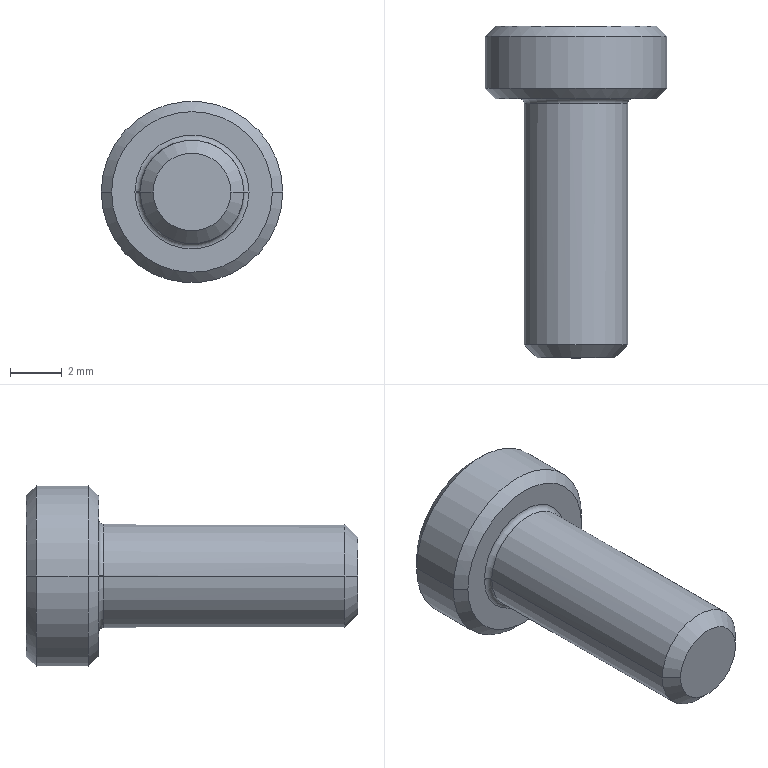Part | SolidWorks | features BaseBody 1 | 1 solid | 32 faces | box 7 x 12.8 x 7 mm | volume 210.469 mm3 | cylinder 18 | cone 6 | plane 4 | torus 4 | commonest cylinder face diameters 1 x8 3.286 x6 4 x2 7 x2
STEP:
#1=CARTESIAN_POINT('',(1970.222,195.3,831.468));
#2=VERTEX_POINT('',#1);
#3=CARTESIAN_POINT('',(1964.022,195.3,831.468));
#4=VERTEX_POINT('',#3);
#5=CARTESIAN_POINT('',(1970.222,195.3,831.468));
#6=CARTESIAN_POINT('',(1970.222,195.3,831.123));
#7=CARTESIAN_POINT('',(1970.174,195.3,830.778));
#8=CARTESIAN_POINT('',(1970.078,195.3,830.441));
#9=CARTESIAN_POINT('',(1969.795,195.3,829.805));
#10=CARTESIAN_POINT('',(1969.349,195.3,829.27));
#11=CARTESIAN_POINT('',(1969.09,195.3,829.035));
#12=CARTESIAN_POINT('',(1968.513,195.3,828.644));
#13=CARTESIAN_POINT('',(1967.852,195.3,828.425));
#14=CARTESIAN_POINT('',(1967.508,195.3,828.362));
#15=CARTESIAN_POINT('',(1966.811,195.3,828.335));
#16=CARTESIAN_POINT('',(1966.134,195.3,828.498));
#17=CARTESIAN_POINT('',(1965.809,195.3,828.627));
#18=CARTESIAN_POINT('',(1965.204,195.3,828.971));
#19=CARTESIAN_POINT('',(1964.715,195.3,829.468));
#20=CARTESIAN_POINT('',(1964.507,195.3,829.749));
#21=CARTESIAN_POINT('',(1964.233,195.3,830.253));
#22=CARTESIAN_POINT('',(1964.082,195.3,830.802));
#23=CARTESIAN_POINT('',(1964.042,195.3,831.022));
#24=CARTESIAN_POINT('',(1964.022,195.3,831.245));
#25=CARTESIAN_POINT('',(1964.022,195.3,831.468));
#26=B_SPLINE_CURVE_WITH_KNOTS('',5,(#5,#6,#7,#8,#9,#10,#11,#12,#13,#14,#15,#16,#17,#18,#19,#20,#21,#22,#23,#24,#25),.UNSPECIFIED.,.F.,.F.,(6,3,3,3,3,3,6),(0.,0.1771,0.3543,0.5314,0.7085,0.8857,1.),.UNSPECIFIED.);
#27=EDGE_CURVE('',#2,#4,#26,.T.);
#28=ORIENTED_EDGE('',*,*,#27,.F.);
#29=CARTESIAN_POINT('',(1967.122,195.3,831.468));
#30=DIRECTION('',(0.,-1.,0.));
#31=DIRECTION('',(0.,0.,-1.));
#32=AXIS2_PLACEMENT_3D('',#29,#30,#31);
#33=CIRCLE('',#32,3.1);
#34=EDGE_CURVE('',#2,#4,#33,.T.);
#35=ORIENTED_EDGE('',*,*,#34,.T.);
#36=EDGE_LOOP('',(#28,#35));
#37=FACE_OUTER_BOUND('',#36,.T.);
#38=CARTESIAN_POINT('',(1964.922,195.3,831.495));
#39=VERTEX_POINT('',#38);
#40=CARTESIAN_POINT('',(1964.922,195.3,831.468));
#41=VERTEX_POINT('',#40);
#42=CARTESIAN_POINT('',(1967.122,195.3,831.468));
#43=DIRECTION('',(0.,-1.,0.));
#44=DIRECTION('',(0.,0.,-1.));
#45=AXIS2_PLACEMENT_3D('',#42,#43,#44);
#46=CIRCLE('',#45,2.2);
#47=EDGE_CURVE('',#39,#41,#46,.T.);
#48=ORIENTED_EDGE('',*,*,#47,.F.);
#49=CARTESIAN_POINT('',(1969.322,195.3,831.468));
#50=VERTEX_POINT('',#49);
#51=CARTESIAN_POINT('',(1967.122,195.3,831.468));
#52=DIRECTION('',(0.,-1.,0.));
#53=DIRECTION('',(0.,0.,-1.));
#54=AXIS2_PLACEMENT_3D('',#51,#52,#53);
#55=CIRCLE('',#54,2.2);
#56=EDGE_CURVE('',#50,#39,#55,.T.);
#57=ORIENTED_EDGE('',*,*,#56,.F.);
#58=CARTESIAN_POINT('',(1969.321,195.3,831.44));
#59=VERTEX_POINT('',#58);
#60=CARTESIAN_POINT('',(1967.122,195.3,831.468));
#61=DIRECTION('',(0.,-1.,0.));
#62=DIRECTION('',(0.,0.,-1.));
#63=AXIS2_PLACEMENT_3D('',#60,#61,#62);
#64=CIRCLE('',#63,2.2);
#65=EDGE_CURVE('',#59,#50,#64,.T.);
#66=ORIENTED_EDGE('',*,*,#65,.F.);
#67=CARTESIAN_POINT('',(1967.122,195.3,831.468));
#68=DIRECTION('',(0.,-1.,0.));
#69=DIRECTION('',(0.,0.,-1.));
#70=AXIS2_PLACEMENT_3D('',#67,#68,#69);
#71=CIRCLE('',#70,2.2);
#72=EDGE_CURVE('',#41,#59,#71,.T.);
#73=ORIENTED_EDGE('',*,*,#72,.F.);
#74=EDGE_LOOP('',(#48,#57,#66,#73));
#75=FACE_BOUND('',#74,.T.);
#76=CARTESIAN_POINT('',(1967.122,195.3,831.468));
#77=DIRECTION('',(0.,-1.,0.));
#78=DIRECTION('',(1.,0.,0.));
#79=AXIS2_PLACEMENT_3D('',#76,#77,#78);
#80=PLANE('',#79);
#81=ADVANCED_FACE('',(#37,#75),#80,.T.);
#82=CARTESIAN_POINT('',(1970.622,195.7,831.468));
#83=VERTEX_POINT('',#82);
#84=CARTESIAN_POINT('',(355522.162,353747.241,831.468));
#85=DIRECTION('',(0.7071,0.7071,0.));
#86=VECTOR('',#85,1000.);
#87=LINE('',#84,#86);
#88=EDGE_CURVE('',#2,#83,#87,.T.);
#89=ORIENTED_EDGE('',*,*,#88,.F.);
#90=ORIENTED_EDGE('',*,*,#27,.T.);
#91=CARTESIAN_POINT('',(1963.622,195.7,831.468));
#92=VERTEX_POINT('',#91);
#93=CARTESIAN_POINT('',(-351587.919,353747.241,831.468));
#94=DIRECTION('',(0.7071,-0.7071,0.));
#95=VECTOR('',#94,1000.);
#96=LINE('',#93,#95);
#97=EDGE_CURVE('',#92,#4,#96,.T.);
#98=ORIENTED_EDGE('',*,*,#97,.F.);
#99=CARTESIAN_POINT('',(1967.122,195.7,831.468));
#100=DIRECTION('',(0.,1.,0.));
#101=DIRECTION('',(0.,0.,1.));
#102=AXIS2_PLACEMENT_3D('',#99,#100,#101);
#103=CIRCLE('',#102,3.5);
#104=EDGE_CURVE('',#83,#92,#103,.T.);
#105=ORIENTED_EDGE('',*,*,#104,.F.);
#106=EDGE_LOOP('',(#89,#90,#98,#105));
#107=FACE_OUTER_BOUND('',#106,.T.);
#108=CARTESIAN_POINT('',(1967.122,195.5,831.468));
#109=DIRECTION('',(0.,1.,0.));
#110=DIRECTION('',(-1.,0.,0.));
#111=AXIS2_PLACEMENT_3D('',#108,#109,#110);
#112=CONICAL_SURFACE('',#111,3.3,0.7854);
#113=ADVANCED_FACE('',(#107),#112,.T.);
#114=ORIENTED_EDGE('',*,*,#97,.T.);
#115=ORIENTED_EDGE('',*,*,#34,.F.);
#116=ORIENTED_EDGE('',*,*,#88,.T.);
#117=CARTESIAN_POINT('',(1967.122,195.7,831.468));
#118=DIRECTION('',(0.,-1.,0.));
#119=DIRECTION('',(0.,0.,1.));
#120=AXIS2_PLACEMENT_3D('',#117,#118,#119);
#121=CIRCLE('',#120,3.5);
#122=EDGE_CURVE('',#83,#92,#121,.T.);
#123=ORIENTED_EDGE('',*,*,#122,.T.);
#124=EDGE_LOOP('',(#114,#115,#116,#123));
#125=FACE_OUTER_BOUND('',#124,.T.);
#126=CARTESIAN_POINT('',(1967.122,195.5,831.468));
#127=DIRECTION('',(0.,1.,0.));
#128=DIRECTION('',(1.,0.,0.));
#129=AXIS2_PLACEMENT_3D('',#126,#127,#128);
#130=CONICAL_SURFACE('',#129,3.3,0.7854);
#131=ADVANCED_FACE('',(#125),#130,.T.);
#132=ORIENTED_EDGE('',*,*,#47,.T.);
#133=CARTESIAN_POINT('',(1965.122,195.1,831.468));
#134=VERTEX_POINT('',#133);
#135=CARTESIAN_POINT('',(1964.922,195.1,831.468));
#136=DIRECTION('',(0.,0.,-1.));
#137=DIRECTION('',(0.,-1.,0.));
#138=AXIS2_PLACEMENT_3D('',#135,#136,#137);
#139=CIRCLE('',#138,0.2);
#140=EDGE_CURVE('',#41,#134,#139,.T.);
#141=ORIENTED_EDGE('',*,*,#140,.T.);
#142=CARTESIAN_POINT('',(1965.122,195.1,831.492));
#143=VERTEX_POINT('',#142);
#144=CARTESIAN_POINT('',(1967.122,195.1,831.468));
#145=DIRECTION('',(0.,-1.,0.));
#146=DIRECTION('',(0.,0.,-1.));
#147=AXIS2_PLACEMENT_3D('',#144,#145,#146);
#148=CIRCLE('',#147,2.);
#149=EDGE_CURVE('',#143,#134,#148,.T.);
#150=ORIENTED_EDGE('',*,*,#149,.F.);
#151=CARTESIAN_POINT('',(1964.922,195.1,831.495));
#152=DIRECTION('',(0.01244,0.,0.9999));
#153=DIRECTION('',(0.,-1.,0.));
#154=AXIS2_PLACEMENT_3D('',#151,#152,#153);
#155=CIRCLE('',#154,0.2);
#156=EDGE_CURVE('',#143,#39,#155,.T.);
#157=ORIENTED_EDGE('',*,*,#156,.T.);
#158=EDGE_LOOP('',(#132,#141,#150,#157));
#159=FACE_OUTER_BOUND('',#158,.T.);
#160=CARTESIAN_POINT('',(1967.122,195.1,831.468));
#161=DIRECTION('',(0.,-1.,0.));
#162=DIRECTION('',(0.9999,0.,-0.01244));
#163=AXIS2_PLACEMENT_3D('',#160,#161,#162);
#164=TOROIDAL_SURFACE('',#163,2.2,0.2);
#165=ADVANCED_FACE('',(#159),#164,.F.);
#166=CARTESIAN_POINT('',(1969.122,195.1,831.468));
#167=VERTEX_POINT('',#166);
#168=CARTESIAN_POINT('',(1967.122,195.1,831.468));
#169=DIRECTION('',(0.,-1.,0.));
#170=DIRECTION('',(0.,0.,-1.));
#171=AXIS2_PLACEMENT_3D('',#168,#169,#170);
#172=CIRCLE('',#171,2.);
#173=EDGE_CURVE('',#167,#143,#172,.T.);
#174=ORIENTED_EDGE('',*,*,#173,.F.);
#175=CARTESIAN_POINT('',(1969.322,195.1,831.468));
#176=DIRECTION('',(0.,0.,1.));
#177=DIRECTION('',(0.,-1.,0.));
#178=AXIS2_PLACEMENT_3D('',#175,#176,#177);
#179=CIRCLE('',#178,0.2);
#180=EDGE_CURVE('',#50,#167,#179,.T.);
#181=ORIENTED_EDGE('',*,*,#180,.F.);
#182=ORIENTED_EDGE('',*,*,#56,.T.);
#183=ORIENTED_EDGE('',*,*,#156,.F.);
#184=EDGE_LOOP('',(#174,#181,#182,#183));
#185=FACE_OUTER_BOUND('',#184,.T.);
#186=CARTESIAN_POINT('',(1967.122,195.1,831.468));
#187=DIRECTION('',(0.,-1.,0.));
#188=DIRECTION('',(-0.9999,0.,0.01244));
#189=AXIS2_PLACEMENT_3D('',#186,#187,#188);
#190=TOROIDAL_SURFACE('',#189,2.2,0.2);
#191=ADVANCED_FACE('',(#185),#190,.F.);
#192=ORIENTED_EDGE('',*,*,#65,.T.);
#193=ORIENTED_EDGE('',*,*,#180,.T.);
#194=CARTESIAN_POINT('',(1969.121,195.1,831.443));
#195=VERTEX_POINT('',#194);
#196=CARTESIAN_POINT('',(1967.122,195.1,831.468));
#197=DIRECTION('',(0.,-1.,0.));
#198=DIRECTION('',(0.,0.,-1.));
#199=AXIS2_PLACEMENT_3D('',#196,#197,#198);
#200=CIRCLE('',#199,2.);
#201=EDGE_CURVE('',#195,#167,#200,.T.);
#202=ORIENTED_EDGE('',*,*,#201,.F.);
#203=CARTESIAN_POINT('',(1969.321,195.1,831.44));
#204=DIRECTION('',(-0.01244,0.,-0.9999));
#205=DIRECTION('',(0.,-1.,0.));
#206=AXIS2_PLACEMENT_3D('',#203,#204,#205);
#207=CIRCLE('',#206,0.2);
#208=EDGE_CURVE('',#195,#59,#207,.T.);
#209=ORIENTED_EDGE('',*,*,#208,.T.);
#210=EDGE_LOOP('',(#192,#193,#202,#209));
#211=FACE_OUTER_BOUND('',#210,.T.);
#212=CARTESIAN_POINT('',(1967.122,195.1,831.468));
#213=DIRECTION('',(0.,-1.,0.));
#214=DIRECTION('',(-0.9999,0.,0.01244));
#215=AXIS2_PLACEMENT_3D('',#212,#213,#214);
#216=TOROIDAL_SURFACE('',#215,2.2,0.2);
#217=ADVANCED_FACE('',(#211),#216,.F.);
#218=CARTESIAN_POINT('',(1967.122,195.1,831.468));
#219=DIRECTION('',(0.,-1.,0.));
#220=DIRECTION('',(0.,0.,-1.));
#221=AXIS2_PLACEMENT_3D('',#218,#219,#220);
#222=CIRCLE('',#221,2.);
#223=EDGE_CURVE('',#134,#195,#222,.T.);
#224=ORIENTED_EDGE('',*,*,#223,.F.);
#225=ORIENTED_EDGE('',*,*,#140,.F.);
#226=ORIENTED_EDGE('',*,*,#72,.T.);
#227=ORIENTED_EDGE('',*,*,#208,.F.);
#228=EDGE_LOOP('',(#224,#225,#226,#227));
#229=FACE_OUTER_BOUND('',#228,.T.);
#230=CARTESIAN_POINT('',(1967.122,195.1,831.468));
#231=DIRECTION('',(0.,-1.,0.));
#232=DIRECTION('',(0.9999,0.,-0.01244));
#233=AXIS2_PLACEMENT_3D('',#230,#231,#232);
#234=TOROIDAL_SURFACE('',#233,2.2,0.2);
#235=ADVANCED_FACE('',(#229),#234,.F.);
#236=ORIENTED_EDGE('',*,*,#104,.T.);
#237=CARTESIAN_POINT('',(1963.622,197.7,831.468));
#238=VERTEX_POINT('',#237);
#239=CARTESIAN_POINT('',(1963.622,198.74,831.468));
#240=DIRECTION('',(0.,-1.,0.));
#241=VECTOR('',#240,1000.);
#242=LINE('',#239,#241);
#243=EDGE_CURVE('',#238,#92,#242,.T.);
#244=ORIENTED_EDGE('',*,*,#243,.F.);
#245=CARTESIAN_POINT('',(1970.622,197.7,831.468));
#246=VERTEX_POINT('',#245);
#247=CARTESIAN_POINT('',(1967.122,197.7,831.468));
#248=DIRECTION('',(0.,1.,0.));
#249=DIRECTION('',(0.,0.,-1.));
#250=AXIS2_PLACEMENT_3D('',#247,#248,#249);
#251=CIRCLE('',#250,3.5);
#252=EDGE_CURVE('',#246,#238,#251,.T.);
#253=ORIENTED_EDGE('',*,*,#252,.F.);
#254=CARTESIAN_POINT('',(1970.622,198.74,831.468));
#255=DIRECTION('',(0.,1.,0.));
#256=VECTOR('',#255,1000.);
#257=LINE('',#254,#256);
#258=EDGE_CURVE('',#83,#246,#257,.T.);
#259=ORIENTED_EDGE('',*,*,#258,.F.);
#260=EDGE_LOOP('',(#236,#244,#253,#259));
#261=FACE_OUTER_BOUND('',#260,.T.);
#262=CARTESIAN_POINT('',(1967.122,198.74,831.468));
#263=DIRECTION('',(0.,-1.,0.));
#264=DIRECTION('',(1.,0.,0.));
#265=AXIS2_PLACEMENT_3D('',#262,#263,#264);
#266=CYLINDRICAL_SURFACE('',#265,3.5);
#267=ADVANCED_FACE('',(#261),#266,.T.);
#268=CARTESIAN_POINT('',(1967.122,197.7,831.468));
#269=DIRECTION('',(0.,-1.,0.));
#270=DIRECTION('',(0.,0.,-1.));
#271=AXIS2_PLACEMENT_3D('',#268,#269,#270);
#272=CIRCLE('',#271,3.5);
#273=EDGE_CURVE('',#246,#238,#272,.T.);
#274=ORIENTED_EDGE('',*,*,#273,.T.);
#275=ORIENTED_EDGE('',*,*,#243,.T.);
#276=ORIENTED_EDGE('',*,*,#122,.F.);
#277=ORIENTED_EDGE('',*,*,#258,.T.);
#278=EDGE_LOOP('',(#274,#275,#276,#277));
#279=FACE_OUTER_BOUND('',#278,.T.);
#280=CARTESIAN_POINT('',(1967.122,198.74,831.468));
#281=DIRECTION('',(0.,-1.,0.));
#282=DIRECTION('',(-1.,0.,0.));
#283=AXIS2_PLACEMENT_3D('',#280,#281,#282);
#284=CYLINDRICAL_SURFACE('',#283,3.5);
#285=ADVANCED_FACE('',(#279),#284,.T.);
#286=CARTESIAN_POINT('',(1965.122,185.8,831.468));
#287=VERTEX_POINT('',#286);
#288=CARTESIAN_POINT('',(1965.122,198.74,831.468));
#289=DIRECTION('',(0.,-1.,0.));
#290=VECTOR('',#289,1000.);
#291=LINE('',#288,#290);
#292=EDGE_CURVE('',#134,#287,#291,.T.);
#293=ORIENTED_EDGE('',*,*,#292,.T.);
#294=CARTESIAN_POINT('',(1969.122,185.8,831.468));
#295=VERTEX_POINT('',#294);
#296=CARTESIAN_POINT('',(1967.122,185.8,831.468));
#297=DIRECTION('',(0.,-1.,0.));
#298=DIRECTION('',(0.,0.,1.));
#299=AXIS2_PLACEMENT_3D('',#296,#297,#298);
#300=CIRCLE('',#299,2.);
#301=EDGE_CURVE('',#295,#287,#300,.T.);
#302=ORIENTED_EDGE('',*,*,#301,.F.);
#303=CARTESIAN_POINT('',(1969.122,198.74,831.468));
#304=DIRECTION('',(0.,1.,0.));
#305=VECTOR('',#304,1000.);
#306=LINE('',#303,#305);
#307=EDGE_CURVE('',#295,#167,#306,.T.);
#308=ORIENTED_EDGE('',*,*,#307,.T.);
#309=ORIENTED_EDGE('',*,*,#173,.T.);
#310=ORIENTED_EDGE('',*,*,#149,.T.);
#311=EDGE_LOOP('',(#293,#302,#308,#309,#310));
#312=FACE_OUTER_BOUND('',#311,.T.);
#313=CARTESIAN_POINT('',(1967.122,198.74,831.468));
#314=DIRECTION('',(0.,-1.,0.));
#315=DIRECTION('',(-1.,0.,0.));
#316=AXIS2_PLACEMENT_3D('',#313,#314,#315);
#317=CYLINDRICAL_SURFACE('',#316,2.);
#318=ADVANCED_FACE('',(#312),#317,.T.);
#319=ORIENTED_EDGE('',*,*,#307,.F.);
#320=CARTESIAN_POINT('',(1967.122,185.8,831.468));
#321=DIRECTION('',(0.,1.,0.));
#322=DIRECTION('',(0.,0.,-1.));
#323=AXIS2_PLACEMENT_3D('',#320,#321,#322);
#324=CIRCLE('',#323,2.);
#325=EDGE_CURVE('',#295,#287,#324,.T.);
#326=ORIENTED_EDGE('',*,*,#325,.T.);
#327=ORIENTED_EDGE('',*,*,#292,.F.);
#328=ORIENTED_EDGE('',*,*,#223,.T.);
#329=ORIENTED_EDGE('',*,*,#201,.T.);
#330=EDGE_LOOP('',(#319,#326,#327,#328,#329));
#331=FACE_OUTER_BOUND('',#330,.T.);
#332=CARTESIAN_POINT('',(1967.122,198.74,831.468));
#333=DIRECTION('',(0.,-1.,0.));
#334=DIRECTION('',(1.,0.,0.));
#335=AXIS2_PLACEMENT_3D('',#332,#333,#334);
#336=CYLINDRICAL_SURFACE('',#335,2.);
#337=ADVANCED_FACE('',(#331),#336,.T.);
#338=CARTESIAN_POINT('',(1970.222,198.1,831.468));
#339=VERTEX_POINT('',#338);
#340=CARTESIAN_POINT('',(355522.162,-353353.841,831.468));
#341=DIRECTION('',(0.7071,-0.7071,0.));
#342=VECTOR('',#341,1000.);
#343=LINE('',#340,#342);
#344=EDGE_CURVE('',#339,#246,#343,.T.);
#345=ORIENTED_EDGE('',*,*,#344,.T.);
#346=ORIENTED_EDGE('',*,*,#252,.T.);
#347=CARTESIAN_POINT('',(1964.022,198.1,831.468));
#348=VERTEX_POINT('',#347);
#349=CARTESIAN_POINT('',(-351587.919,-353353.841,831.468));
#350=DIRECTION('',(0.7071,0.7071,0.));
#351=VECTOR('',#350,1000.);
#352=LINE('',#349,#351);
#353=EDGE_CURVE('',#238,#348,#352,.T.);
#354=ORIENTED_EDGE('',*,*,#353,.T.);
#355=CARTESIAN_POINT('',(1967.122,198.1,831.468));
#356=DIRECTION('',(0.,1.,0.));
#357=DIRECTION('',(0.,0.,-1.));
#358=AXIS2_PLACEMENT_3D('',#355,#356,#357);
#359=CIRCLE('',#358,3.1);
#360=EDGE_CURVE('',#339,#348,#359,.T.);
#361=ORIENTED_EDGE('',*,*,#360,.F.);
#362=EDGE_LOOP('',(#345,#346,#354,#361));
#363=FACE_OUTER_BOUND('',#362,.T.);
#364=CARTESIAN_POINT('',(1967.122,197.9,831.468));
#365=DIRECTION('',(0.,-1.,0.));
#366=DIRECTION('',(1.,0.,0.));
#367=AXIS2_PLACEMENT_3D('',#364,#365,#366);
#368=CONICAL_SURFACE('',#367,3.3,0.7854);
#369=ADVANCED_FACE('',(#363),#368,.T.);
#370=ORIENTED_EDGE('',*,*,#353,.F.);
#371=ORIENTED_EDGE('',*,*,#273,.F.);
#372=ORIENTED_EDGE('',*,*,#344,.F.);
#373=CARTESIAN_POINT('',(1967.122,198.1,831.468));
#374=DIRECTION('',(0.,-1.,0.));
#375=DIRECTION('',(0.,0.,-1.));
#376=AXIS2_PLACEMENT_3D('',#373,#374,#375);
#377=CIRCLE('',#376,3.1);
#378=EDGE_CURVE('',#339,#348,#377,.T.);
#379=ORIENTED_EDGE('',*,*,#378,.T.);
#380=EDGE_LOOP('',(#370,#371,#372,#379));
#381=FACE_OUTER_BOUND('',#380,.T.);
#382=CARTESIAN_POINT('',(1967.122,197.9,831.468));
#383=DIRECTION('',(0.,-1.,0.));
#384=DIRECTION('',(-1.,0.,0.));
#385=AXIS2_PLACEMENT_3D('',#382,#383,#384);
#386=CONICAL_SURFACE('',#385,3.3,0.7854);
#387=ADVANCED_FACE('',(#381),#386,.T.);
#388=CARTESIAN_POINT('',(1965.622,185.3,831.468));
#389=VERTEX_POINT('',#388);
#390=CARTESIAN_POINT('',(-351587.144,353738.066,831.468));
#391=DIRECTION('',(-0.7071,0.7071,0.));
#392=VECTOR('',#391,1000.);
#393=LINE('',#390,#392);
#394=EDGE_CURVE('',#389,#287,#393,.T.);
#395=ORIENTED_EDGE('',*,*,#394,.F.);
#396=CARTESIAN_POINT('',(1968.622,185.3,831.468));
#397=VERTEX_POINT('',#396);
#398=CARTESIAN_POINT('',(1967.122,185.3,831.468));
#399=DIRECTION('',(0.,-1.,0.));
#400=DIRECTION('',(0.,0.,1.));
#401=AXIS2_PLACEMENT_3D('',#398,#399,#400);
#402=CIRCLE('',#401,1.5);
#403=EDGE_CURVE('',#397,#389,#402,.T.);
#404=ORIENTED_EDGE('',*,*,#403,.F.);
#405=CARTESIAN_POINT('',(355521.387,353738.066,831.468));
#406=DIRECTION('',(-0.7071,-0.7071,0.));
#407=VECTOR('',#406,1000.);
#408=LINE('',#405,#407);
#409=EDGE_CURVE('',#295,#397,#408,.T.);
#410=ORIENTED_EDGE('',*,*,#409,.F.);
#411=ORIENTED_EDGE('',*,*,#301,.T.);
#412=EDGE_LOOP('',(#395,#404,#410,#411));
#413=FACE_OUTER_BOUND('',#412,.T.);
#414=CARTESIAN_POINT('',(1967.122,185.55,831.468));
#415=DIRECTION('',(0.,1.,0.));
#416=DIRECTION('',(1.,0.,0.));
#417=AXIS2_PLACEMENT_3D('',#414,#415,#416);
#418=CONICAL_SURFACE('',#417,1.75,0.7854);
#419=ADVANCED_FACE('',(#413),#418,.T.);
#420=ORIENTED_EDGE('',*,*,#409,.T.);
#421=CARTESIAN_POINT('',(1967.122,185.3,831.468));
#422=DIRECTION('',(0.,1.,0.));
#423=DIRECTION('',(0.,0.,1.));
#424=AXIS2_PLACEMENT_3D('',#421,#422,#423);
#425=CIRCLE('',#424,1.5);
#426=EDGE_CURVE('',#397,#389,#425,.T.);
#427=ORIENTED_EDGE('',*,*,#426,.T.);
#428=ORIENTED_EDGE('',*,*,#394,.T.);
#429=ORIENTED_EDGE('',*,*,#325,.F.);
#430=EDGE_LOOP('',(#420,#427,#428,#429));
#431=FACE_OUTER_BOUND('',#430,.T.);
#432=CARTESIAN_POINT('',(1967.122,185.55,831.468));
#433=DIRECTION('',(0.,1.,0.));
#434=DIRECTION('',(-1.,0.,0.));
#435=AXIS2_PLACEMENT_3D('',#432,#433,#434);
#436=CONICAL_SURFACE('',#435,1.75,0.7854);
#437=ADVANCED_FACE('',(#431),#436,.T.);
#438=ORIENTED_EDGE('',*,*,#378,.F.);
#439=ORIENTED_EDGE('',*,*,#360,.T.);
#440=EDGE_LOOP('',(#438,#439));
#441=FACE_OUTER_BOUND('',#440,.T.);
#442=CARTESIAN_POINT('',(1967.685,198.1,829.725));
#443=VERTEX_POINT('',#442);
#444=CARTESIAN_POINT('',(1966.558,198.1,829.725));
#445=VERTEX_POINT('',#444);
#446=CARTESIAN_POINT('',(1967.122,198.1,828.181));
#447=DIRECTION('',(0.,-1.,0.));
#448=DIRECTION('',(0.,0.,-1.));
#449=AXIS2_PLACEMENT_3D('',#446,#447,#448);
#450=CIRCLE('',#449,1.643);
#451=EDGE_CURVE('',#443,#445,#450,.T.);
#452=ORIENTED_EDGE('',*,*,#451,.F.);
#453=CARTESIAN_POINT('',(1968.349,198.1,830.108));
#454=VERTEX_POINT('',#453);
#455=CARTESIAN_POINT('',(1967.857,198.1,830.195));
#456=DIRECTION('',(0.,-1.,0.));
#457=DIRECTION('',(0.,0.,-1.));
#458=AXIS2_PLACEMENT_3D('',#455,#456,#457);
#459=CIRCLE('',#458,0.5);
#460=EDGE_CURVE('',#443,#454,#459,.T.);
#461=ORIENTED_EDGE('',*,*,#460,.T.);
#462=CARTESIAN_POINT('',(1968.913,198.1,831.084));
#463=VERTEX_POINT('',#462);
#464=CARTESIAN_POINT('',(1969.967,198.1,829.825));
#465=DIRECTION('',(0.,-1.,0.));
#466=DIRECTION('',(0.,0.,-1.));
#467=AXIS2_PLACEMENT_3D('',#464,#465,#466);
#468=CIRCLE('',#467,1.643);
#469=EDGE_CURVE('',#463,#454,#468,.T.);
#470=ORIENTED_EDGE('',*,*,#469,.F.);
#471=CARTESIAN_POINT('',(1969.092,198.1,831.468));
#472=VERTEX_POINT('',#471);
#473=CARTESIAN_POINT('',(1968.592,198.1,831.468));
#474=DIRECTION('',(0.,-1.,0.));
#475=DIRECTION('',(0.,0.,-1.));
#476=AXIS2_PLACEMENT_3D('',#473,#474,#475);
#477=CIRCLE('',#476,0.5);
#478=EDGE_CURVE('',#463,#472,#477,.T.);
#479=ORIENTED_EDGE('',*,*,#478,.T.);
#480=CARTESIAN_POINT('',(1968.913,198.1,831.851));
#481=VERTEX_POINT('',#480);
#482=CARTESIAN_POINT('',(1968.592,198.1,831.468));
#483=DIRECTION('',(0.,-1.,0.));
#484=DIRECTION('',(0.,0.,-1.));
#485=AXIS2_PLACEMENT_3D('',#482,#483,#484);
#486=CIRCLE('',#485,0.5);
#487=EDGE_CURVE('',#472,#481,#486,.T.);
#488=ORIENTED_EDGE('',*,*,#487,.T.);
#489=CARTESIAN_POINT('',(1968.349,198.1,832.827));
#490=VERTEX_POINT('',#489);
#491=CARTESIAN_POINT('',(1969.967,198.1,833.111));
#492=DIRECTION('',(0.,-1.,0.));
#493=DIRECTION('',(0.,0.,-1.));
#494=AXIS2_PLACEMENT_3D('',#491,#492,#493);
#495=CIRCLE('',#494,1.643);
#496=EDGE_CURVE('',#490,#481,#495,.T.);
#497=ORIENTED_EDGE('',*,*,#496,.F.);
#498=CARTESIAN_POINT('',(1967.685,198.1,833.21));
#499=VERTEX_POINT('',#498);
#500=CARTESIAN_POINT('',(1967.857,198.1,832.741));
#501=DIRECTION('',(0.,-1.,0.));
#502=DIRECTION('',(0.,0.,-1.));
#503=AXIS2_PLACEMENT_3D('',#500,#501,#502);
#504=CIRCLE('',#503,0.5);
#505=EDGE_CURVE('',#490,#499,#504,.T.);
#506=ORIENTED_EDGE('',*,*,#505,.T.);
#507=CARTESIAN_POINT('',(1966.558,198.1,833.21));
#508=VERTEX_POINT('',#507);
#509=CARTESIAN_POINT('',(1967.122,198.1,834.754));
#510=DIRECTION('',(0.,-1.,0.));
#511=DIRECTION('',(0.,0.,-1.));
#512=AXIS2_PLACEMENT_3D('',#509,#510,#511);
#513=CIRCLE('',#512,1.643);
#514=EDGE_CURVE('',#508,#499,#513,.T.);
#515=ORIENTED_EDGE('',*,*,#514,.F.);
#516=CARTESIAN_POINT('',(1965.894,198.1,832.827));
#517=VERTEX_POINT('',#516);
#518=CARTESIAN_POINT('',(1966.387,198.1,832.741));
#519=DIRECTION('',(0.,-1.,0.));
#520=DIRECTION('',(0.,0.,-1.));
#521=AXIS2_PLACEMENT_3D('',#518,#519,#520);
#522=CIRCLE('',#521,0.5);
#523=EDGE_CURVE('',#508,#517,#522,.T.);
#524=ORIENTED_EDGE('',*,*,#523,.T.);
#525=CARTESIAN_POINT('',(1965.331,198.1,831.851));
#526=VERTEX_POINT('',#525);
#527=CARTESIAN_POINT('',(1964.276,198.1,833.111));
#528=DIRECTION('',(0.,-1.,0.));
#529=DIRECTION('',(0.,0.,-1.));
#530=AXIS2_PLACEMENT_3D('',#527,#528,#529);
#531=CIRCLE('',#530,1.643);
#532=EDGE_CURVE('',#526,#517,#531,.T.);
#533=ORIENTED_EDGE('',*,*,#532,.F.);
#534=CARTESIAN_POINT('',(1965.152,198.1,831.468));
#535=VERTEX_POINT('',#534);
#536=CARTESIAN_POINT('',(1965.652,198.1,831.468));
#537=DIRECTION('',(0.,-1.,0.));
#538=DIRECTION('',(0.,0.,-1.));
#539=AXIS2_PLACEMENT_3D('',#536,#537,#538);
#540=CIRCLE('',#539,0.5);
#541=EDGE_CURVE('',#526,#535,#540,.T.);
#542=ORIENTED_EDGE('',*,*,#541,.T.);
#543=CARTESIAN_POINT('',(1965.331,198.1,831.084));
#544=VERTEX_POINT('',#543);
#545=CARTESIAN_POINT('',(1965.652,198.1,831.468));
#546=DIRECTION('',(0.,-1.,0.));
#547=DIRECTION('',(0.,0.,-1.));
#548=AXIS2_PLACEMENT_3D('',#545,#546,#547);
#549=CIRCLE('',#548,0.5);
#550=EDGE_CURVE('',#535,#544,#549,.T.);
#551=ORIENTED_EDGE('',*,*,#550,.T.);
#552=CARTESIAN_POINT('',(1965.894,198.1,830.108));
#553=VERTEX_POINT('',#552);
#554=CARTESIAN_POINT('',(1964.276,198.1,829.825));
#555=DIRECTION('',(0.,-1.,0.));
#556=DIRECTION('',(0.,0.,-1.));
#557=AXIS2_PLACEMENT_3D('',#554,#555,#556);
#558=CIRCLE('',#557,1.643);
#559=EDGE_CURVE('',#553,#544,#558,.T.);
#560=ORIENTED_EDGE('',*,*,#559,.F.);
#561=CARTESIAN_POINT('',(1966.387,198.1,830.195));
#562=DIRECTION('',(0.,-1.,0.));
#563=DIRECTION('',(0.,0.,-1.));
#564=AXIS2_PLACEMENT_3D('',#561,#562,#563);
#565=CIRCLE('',#564,0.5);
#566=EDGE_CURVE('',#553,#445,#565,.T.);
#567=ORIENTED_EDGE('',*,*,#566,.T.);
#568=EDGE_LOOP('',(#452,#461,#470,#479,#488,#497,#506,#515,#524,#533,#542,#551,#560,#567));
#569=FACE_BOUND('',#568,.T.);
#570=CARTESIAN_POINT('',(1967.122,198.1,831.468));
#571=DIRECTION('',(0.,-1.,0.));
#572=DIRECTION('',(1.,0.,0.));
#573=AXIS2_PLACEMENT_3D('',#570,#571,#572);
#574=PLANE('',#573);
#575=ADVANCED_FACE('',(#441,#569),#574,.F.);
#576=ORIENTED_EDGE('',*,*,#403,.T.);
#577=ORIENTED_EDGE('',*,*,#426,.F.);
#578=EDGE_LOOP('',(#576,#577));
#579=FACE_OUTER_BOUND('',#578,.T.);
#580=CARTESIAN_POINT('',(1967.122,185.3,831.468));
#581=DIRECTION('',(0.,-1.,0.));
#582=DIRECTION('',(1.,0.,0.));
#583=AXIS2_PLACEMENT_3D('',#580,#581,#582);
#584=PLANE('',#583);
#585=ADVANCED_FACE('',(#579),#584,.T.);
#586=CARTESIAN_POINT('',(1966.558,196.3,829.725));
#587=VERTEX_POINT('',#586);
#588=CARTESIAN_POINT('',(1967.685,196.3,829.725));
#589=VERTEX_POINT('',#588);
#590=CARTESIAN_POINT('',(1967.122,196.3,828.181));
#591=DIRECTION('',(0.,1.,0.));
#592=DIRECTION('',(0.,0.,-1.));
#593=AXIS2_PLACEMENT_3D('',#590,#591,#592);
#594=CIRCLE('',#593,1.643);
#595=EDGE_CURVE('',#587,#589,#594,.T.);
#596=ORIENTED_EDGE('',*,*,#595,.T.);
#597=CARTESIAN_POINT('',(1967.685,196.3,829.725));
#598=DIRECTION('',(0.,1.,0.));
#599=VECTOR('',#598,1000.);
#600=LINE('',#597,#599);
#601=EDGE_CURVE('',#589,#443,#600,.T.);
#602=ORIENTED_EDGE('',*,*,#601,.T.);
#603=ORIENTED_EDGE('',*,*,#451,.T.);
#604=CARTESIAN_POINT('',(1966.558,196.3,829.725));
#605=DIRECTION('',(0.,1.,0.));
#606=VECTOR('',#605,1000.);
#607=LINE('',#604,#606);
#608=EDGE_CURVE('',#587,#445,#607,.T.);
#609=ORIENTED_EDGE('',*,*,#608,.F.);
#610=EDGE_LOOP('',(#596,#602,#603,#609));
#611=FACE_OUTER_BOUND('',#610,.T.);
#612=CARTESIAN_POINT('',(1967.122,196.3,828.181));
#613=DIRECTION('',(0.,-1.,0.));
#614=DIRECTION('',(-1.,0.,0.));
#615=AXIS2_PLACEMENT_3D('',#612,#613,#614);
#616=CYLINDRICAL_SURFACE('',#615,1.643);
#617=ADVANCED_FACE('',(#611),#616,.T.);
#618=CARTESIAN_POINT('',(1968.349,196.3,830.108));
#619=VERTEX_POINT('',#618);
#620=CARTESIAN_POINT('',(1967.857,196.3,830.195));
#621=DIRECTION('',(0.,-1.,0.));
#622=DIRECTION('',(0.,0.,-1.));
#623=AXIS2_PLACEMENT_3D('',#620,#621,#622);
#624=CIRCLE('',#623,0.5);
#625=EDGE_CURVE('',#589,#619,#624,.T.);
#626=ORIENTED_EDGE('',*,*,#625,.T.);
#627=CARTESIAN_POINT('',(1968.349,196.3,830.108));
#628=DIRECTION('',(0.,1.,0.));
#629=VECTOR('',#628,1000.);
#630=LINE('',#627,#629);
#631=EDGE_CURVE('',#619,#454,#630,.T.);
#632=ORIENTED_EDGE('',*,*,#631,.T.);
#633=ORIENTED_EDGE('',*,*,#460,.F.);
#634=ORIENTED_EDGE('',*,*,#601,.F.);
#635=EDGE_LOOP('',(#626,#632,#633,#634));
#636=FACE_OUTER_BOUND('',#635,.T.);
#637=CARTESIAN_POINT('',(1967.857,196.3,830.195));
#638=DIRECTION('',(0.,-1.,0.));
#639=DIRECTION('',(1.,0.,0.));
#640=AXIS2_PLACEMENT_3D('',#637,#638,#639);
#641=CYLINDRICAL_SURFACE('',#640,0.5);
#642=ADVANCED_FACE('',(#636),#641,.F.);
#643=CARTESIAN_POINT('',(1968.913,196.3,831.084));
#644=VERTEX_POINT('',#643);
#645=CARTESIAN_POINT('',(1969.967,196.3,829.825));
#646=DIRECTION('',(0.,1.,0.));
#647=DIRECTION('',(0.,0.,-1.));
#648=AXIS2_PLACEMENT_3D('',#645,#646,#647);
#649=CIRCLE('',#648,1.643);
#650=EDGE_CURVE('',#619,#644,#649,.T.);
#651=ORIENTED_EDGE('',*,*,#650,.T.);
#652=CARTESIAN_POINT('',(1968.913,196.3,831.084));
#653=DIRECTION('',(0.,1.,0.));
#654=VECTOR('',#653,1000.);
#655=LINE('',#652,#654);
#656=EDGE_CURVE('',#644,#463,#655,.T.);
#657=ORIENTED_EDGE('',*,*,#656,.T.);
#658=ORIENTED_EDGE('',*,*,#469,.T.);
#659=ORIENTED_EDGE('',*,*,#631,.F.);
#660=EDGE_LOOP('',(#651,#657,#658,#659));
#661=FACE_OUTER_BOUND('',#660,.T.);
#662=CARTESIAN_POINT('',(1969.967,196.3,829.825));
#663=DIRECTION('',(0.,-1.,0.));
#664=DIRECTION('',(-1.,0.,0.));
#665=AXIS2_PLACEMENT_3D('',#662,#663,#664);
#666=CYLINDRICAL_SURFACE('',#665,1.643);
#667=ADVANCED_FACE('',(#661),#666,.T.);
#668=ORIENTED_EDGE('',*,*,#478,.F.);
#669=ORIENTED_EDGE('',*,*,#656,.F.);
#670=CARTESIAN_POINT('',(1969.092,196.3,831.468));
#671=VERTEX_POINT('',#670);
#672=CARTESIAN_POINT('',(1968.592,196.3,831.468));
#673=DIRECTION('',(0.,-1.,0.));
#674=DIRECTION('',(0.,0.,-1.));
#675=AXIS2_PLACEMENT_3D('',#672,#673,#674);
#676=CIRCLE('',#675,0.5);
#677=EDGE_CURVE('',#644,#671,#676,.T.);
#678=ORIENTED_EDGE('',*,*,#677,.T.);
#679=CARTESIAN_POINT('',(1969.092,196.3,831.468));
#680=DIRECTION('',(0.,-1.,0.));
#681=VECTOR('',#680,1000.);
#682=LINE('',#679,#681);
#683=EDGE_CURVE('',#472,#671,#682,.T.);
#684=ORIENTED_EDGE('',*,*,#683,.F.);
#685=EDGE_LOOP('',(#668,#669,#678,#684));
#686=FACE_OUTER_BOUND('',#685,.T.);
#687=CARTESIAN_POINT('',(1968.592,196.3,831.468));
#688=DIRECTION('',(0.,-1.,0.));
#689=DIRECTION('',(1.,0.,0.));
#690=AXIS2_PLACEMENT_3D('',#687,#688,#689);
#691=CYLINDRICAL_SURFACE('',#690,0.5);
#692=ADVANCED_FACE('',(#686),#691,.F.);
#693=CARTESIAN_POINT('',(1968.913,196.3,831.851));
#694=VERTEX_POINT('',#693);
#695=CARTESIAN_POINT('',(1968.592,196.3,831.468));
#696=DIRECTION('',(0.,-1.,0.));
#697=DIRECTION('',(0.,0.,-1.));
#698=AXIS2_PLACEMENT_3D('',#695,#696,#697);
#699=CIRCLE('',#698,0.5);
#700=EDGE_CURVE('',#671,#694,#699,.T.);
#701=ORIENTED_EDGE('',*,*,#700,.T.);
#702=CARTESIAN_POINT('',(1968.913,196.3,831.851));
#703=DIRECTION('',(0.,1.,0.));
#704=VECTOR('',#703,1000.);
#705=LINE('',#702,#704);
#706=EDGE_CURVE('',#694,#481,#705,.T.);
#707=ORIENTED_EDGE('',*,*,#706,.T.);
#708=ORIENTED_EDGE('',*,*,#487,.F.);
#709=ORIENTED_EDGE('',*,*,#683,.T.);
#710=EDGE_LOOP('',(#701,#707,#708,#709));
#711=FACE_OUTER_BOUND('',#710,.T.);
#712=CARTESIAN_POINT('',(1968.592,196.3,831.468));
#713=DIRECTION('',(0.,-1.,0.));
#714=DIRECTION('',(-1.,0.,0.));
#715=AXIS2_PLACEMENT_3D('',#712,#713,#714);
#716=CYLINDRICAL_SURFACE('',#715,0.5);
#717=ADVANCED_FACE('',(#711),#716,.F.);
#718=CARTESIAN_POINT('',(1968.349,196.3,832.827));
#719=VERTEX_POINT('',#718);
#720=CARTESIAN_POINT('',(1969.967,196.3,833.111));
#721=DIRECTION('',(0.,1.,0.));
#722=DIRECTION('',(0.,0.,-1.));
#723=AXIS2_PLACEMENT_3D('',#720,#721,#722);
#724=CIRCLE('',#723,1.643);
#725=EDGE_CURVE('',#694,#719,#724,.T.);
#726=ORIENTED_EDGE('',*,*,#725,.T.);
#727=CARTESIAN_POINT('',(1968.349,196.3,832.827));
#728=DIRECTION('',(0.,1.,0.));
#729=VECTOR('',#728,1000.);
#730=LINE('',#727,#729);
#731=EDGE_CURVE('',#719,#490,#730,.T.);
#732=ORIENTED_EDGE('',*,*,#731,.T.);
#733=ORIENTED_EDGE('',*,*,#496,.T.);
#734=ORIENTED_EDGE('',*,*,#706,.F.);
#735=EDGE_LOOP('',(#726,#732,#733,#734));
#736=FACE_OUTER_BOUND('',#735,.T.);
#737=CARTESIAN_POINT('',(1969.967,196.3,833.111));
#738=DIRECTION('',(0.,-1.,0.));
#739=DIRECTION('',(1.,0.,0.));
#740=AXIS2_PLACEMENT_3D('',#737,#738,#739);
#741=CYLINDRICAL_SURFACE('',#740,1.643);
#742=ADVANCED_FACE('',(#736),#741,.T.);
#743=CARTESIAN_POINT('',(1967.685,196.3,833.21));
#744=VERTEX_POINT('',#743);
#745=CARTESIAN_POINT('',(1967.857,196.3,832.741));
#746=DIRECTION('',(0.,-1.,0.));
#747=DIRECTION('',(0.,0.,-1.));
#748=AXIS2_PLACEMENT_3D('',#745,#746,#747);
#749=CIRCLE('',#748,0.5);
#750=EDGE_CURVE('',#719,#744,#749,.T.);
#751=ORIENTED_EDGE('',*,*,#750,.T.);
#752=CARTESIAN_POINT('',(1967.685,196.3,833.21));
#753=DIRECTION('',(0.,1.,0.));
#754=VECTOR('',#753,1000.);
#755=LINE('',#752,#754);
#756=EDGE_CURVE('',#744,#499,#755,.T.);
#757=ORIENTED_EDGE('',*,*,#756,.T.);
#758=ORIENTED_EDGE('',*,*,#505,.F.);
#759=ORIENTED_EDGE('',*,*,#731,.F.);
#760=EDGE_LOOP('',(#751,#757,#758,#759));
#761=FACE_OUTER_BOUND('',#760,.T.);
#762=CARTESIAN_POINT('',(1967.857,196.3,832.741));
#763=DIRECTION('',(0.,-1.,0.));
#764=DIRECTION('',(-1.,0.,0.));
#765=AXIS2_PLACEMENT_3D('',#762,#763,#764);
#766=CYLINDRICAL_SURFACE('',#765,0.5);
#767=ADVANCED_FACE('',(#761),#766,.F.);
#768=CARTESIAN_POINT('',(1966.558,196.3,833.21));
#769=VERTEX_POINT('',#768);
#770=CARTESIAN_POINT('',(1967.122,196.3,834.754));
#771=DIRECTION('',(0.,1.,0.));
#772=DIRECTION('',(0.,0.,-1.));
#773=AXIS2_PLACEMENT_3D('',#770,#771,#772);
#774=CIRCLE('',#773,1.643);
#775=EDGE_CURVE('',#744,#769,#774,.T.);
#776=ORIENTED_EDGE('',*,*,#775,.T.);
#777=CARTESIAN_POINT('',(1966.558,196.3,833.21));
#778=DIRECTION('',(0.,1.,0.));
#779=VECTOR('',#778,1000.);
#780=LINE('',#777,#779);
#781=EDGE_CURVE('',#769,#508,#780,.T.);
#782=ORIENTED_EDGE('',*,*,#781,.T.);
#783=ORIENTED_EDGE('',*,*,#514,.T.);
#784=ORIENTED_EDGE('',*,*,#756,.F.);
#785=EDGE_LOOP('',(#776,#782,#783,#784));
#786=FACE_OUTER_BOUND('',#785,.T.);
#787=CARTESIAN_POINT('',(1967.122,196.3,834.754));
#788=DIRECTION('',(0.,-1.,0.));
#789=DIRECTION('',(1.,0.,0.));
#790=AXIS2_PLACEMENT_3D('',#787,#788,#789);
#791=CYLINDRICAL_SURFACE('',#790,1.643);
#792=ADVANCED_FACE('',(#786),#791,.T.);
#793=CARTESIAN_POINT('',(1965.894,196.3,832.827));
#794=VERTEX_POINT('',#793);
#795=CARTESIAN_POINT('',(1966.387,196.3,832.741));
#796=DIRECTION('',(0.,-1.,0.));
#797=DIRECTION('',(0.,0.,-1.));
#798=AXIS2_PLACEMENT_3D('',#795,#796,#797);
#799=CIRCLE('',#798,0.5);
#800=EDGE_CURVE('',#769,#794,#799,.T.);
#801=ORIENTED_EDGE('',*,*,#800,.T.);
#802=CARTESIAN_POINT('',(1965.894,196.3,832.827));
#803=DIRECTION('',(0.,1.,0.));
#804=VECTOR('',#803,1000.);
#805=LINE('',#802,#804);
#806=EDGE_CURVE('',#794,#517,#805,.T.);
#807=ORIENTED_EDGE('',*,*,#806,.T.);
#808=ORIENTED_EDGE('',*,*,#523,.F.);
#809=ORIENTED_EDGE('',*,*,#781,.F.);
#810=EDGE_LOOP('',(#801,#807,#808,#809));
#811=FACE_OUTER_BOUND('',#810,.T.);
#812=CARTESIAN_POINT('',(1966.387,196.3,832.741));
#813=DIRECTION('',(0.,-1.,0.));
#814=DIRECTION('',(-1.,0.,0.));
#815=AXIS2_PLACEMENT_3D('',#812,#813,#814);
#816=CYLINDRICAL_SURFACE('',#815,0.5);
#817=ADVANCED_FACE('',(#811),#816,.F.);
#818=CARTESIAN_POINT('',(1965.331,196.3,831.851));
#819=VERTEX_POINT('',#818);
#820=CARTESIAN_POINT('',(1964.276,196.3,833.111));
#821=DIRECTION('',(0.,1.,0.));
#822=DIRECTION('',(0.,0.,-1.));
#823=AXIS2_PLACEMENT_3D('',#820,#821,#822);
#824=CIRCLE('',#823,1.643);
#825=EDGE_CURVE('',#794,#819,#824,.T.);
#826=ORIENTED_EDGE('',*,*,#825,.T.);
#827=CARTESIAN_POINT('',(1965.331,196.3,831.851));
#828=DIRECTION('',(0.,1.,0.));
#829=VECTOR('',#828,1000.);
#830=LINE('',#827,#829);
#831=EDGE_CURVE('',#819,#526,#830,.T.);
#832=ORIENTED_EDGE('',*,*,#831,.T.);
#833=ORIENTED_EDGE('',*,*,#532,.T.);
#834=ORIENTED_EDGE('',*,*,#806,.F.);
#835=EDGE_LOOP('',(#826,#832,#833,#834));
#836=FACE_OUTER_BOUND('',#835,.T.);
#837=CARTESIAN_POINT('',(1964.276,196.3,833.111));
#838=DIRECTION('',(0.,-1.,0.));
#839=DIRECTION('',(1.,0.,0.));
#840=AXIS2_PLACEMENT_3D('',#837,#838,#839);
#841=CYLINDRICAL_SURFACE('',#840,1.643);
#842=ADVANCED_FACE('',(#836),#841,.T.);
#843=ORIENTED_EDGE('',*,*,#541,.F.);
#844=ORIENTED_EDGE('',*,*,#831,.F.);
#845=CARTESIAN_POINT('',(1965.152,196.3,831.468));
#846=VERTEX_POINT('',#845);
#847=CARTESIAN_POINT('',(1965.652,196.3,831.468));
#848=DIRECTION('',(0.,-1.,0.));
#849=DIRECTION('',(0.,0.,-1.));
#850=AXIS2_PLACEMENT_3D('',#847,#848,#849);
#851=CIRCLE('',#850,0.5);
#852=EDGE_CURVE('',#819,#846,#851,.T.);
#853=ORIENTED_EDGE('',*,*,#852,.T.);
#854=CARTESIAN_POINT('',(1965.152,196.3,831.468));
#855=DIRECTION('',(0.,1.,0.));
#856=VECTOR('',#855,1000.);
#857=LINE('',#854,#856);
#858=EDGE_CURVE('',#846,#535,#857,.T.);
#859=ORIENTED_EDGE('',*,*,#858,.T.);
#860=EDGE_LOOP('',(#843,#844,#853,#859));
#861=FACE_OUTER_BOUND('',#860,.T.);
#862=CARTESIAN_POINT('',(1965.652,196.3,831.468));
#863=DIRECTION('',(0.,-1.,0.));
#864=DIRECTION('',(-1.,0.,0.));
#865=AXIS2_PLACEMENT_3D('',#862,#863,#864);
#866=CYLINDRICAL_SURFACE('',#865,0.5);
#867=ADVANCED_FACE('',(#861),#866,.F.);
#868=CARTESIAN_POINT('',(1965.331,196.3,831.084));
#869=VERTEX_POINT('',#868);
#870=CARTESIAN_POINT('',(1965.652,196.3,831.468));
#871=DIRECTION('',(0.,-1.,0.));
#872=DIRECTION('',(0.,0.,-1.));
#873=AXIS2_PLACEMENT_3D('',#870,#871,#872);
#874=CIRCLE('',#873,0.5);
#875=EDGE_CURVE('',#846,#869,#874,.T.);
#876=ORIENTED_EDGE('',*,*,#875,.T.);
#877=CARTESIAN_POINT('',(1965.331,196.3,831.084));
#878=DIRECTION('',(0.,1.,0.));
#879=VECTOR('',#878,1000.);
#880=LINE('',#877,#879);
#881=EDGE_CURVE('',#869,#544,#880,.T.);
#882=ORIENTED_EDGE('',*,*,#881,.T.);
#883=ORIENTED_EDGE('',*,*,#550,.F.);
#884=ORIENTED_EDGE('',*,*,#858,.F.);
#885=EDGE_LOOP('',(#876,#882,#883,#884));
#886=FACE_OUTER_BOUND('',#885,.T.);
#887=CARTESIAN_POINT('',(1965.652,196.3,831.468));
#888=DIRECTION('',(0.,-1.,0.));
#889=DIRECTION('',(1.,0.,0.));
#890=AXIS2_PLACEMENT_3D('',#887,#888,#889);
#891=CYLINDRICAL_SURFACE('',#890,0.5);
#892=ADVANCED_FACE('',(#886),#891,.F.);
#893=ORIENTED_EDGE('',*,*,#559,.T.);
#894=ORIENTED_EDGE('',*,*,#881,.F.);
#895=CARTESIAN_POINT('',(1965.894,196.3,830.108));
#896=VERTEX_POINT('',#895);
#897=CARTESIAN_POINT('',(1964.276,196.3,829.825));
#898=DIRECTION('',(0.,1.,0.));
#899=DIRECTION('',(0.,0.,-1.));
#900=AXIS2_PLACEMENT_3D('',#897,#898,#899);
#901=CIRCLE('',#900,1.643);
#902=EDGE_CURVE('',#869,#896,#901,.T.);
#903=ORIENTED_EDGE('',*,*,#902,.T.);
#904=CARTESIAN_POINT('',(1965.894,196.3,830.108));
#905=DIRECTION('',(0.,1.,0.));
#906=VECTOR('',#905,1000.);
#907=LINE('',#904,#906);
#908=EDGE_CURVE('',#896,#553,#907,.T.);
#909=ORIENTED_EDGE('',*,*,#908,.T.);
#910=EDGE_LOOP('',(#893,#894,#903,#909));
#911=FACE_OUTER_BOUND('',#910,.T.);
#912=CARTESIAN_POINT('',(1964.276,196.3,829.825));
#913=DIRECTION('',(0.,-1.,0.));
#914=DIRECTION('',(-1.,0.,0.));
#915=AXIS2_PLACEMENT_3D('',#912,#913,#914);
#916=CYLINDRICAL_SURFACE('',#915,1.643);
#917=ADVANCED_FACE('',(#911),#916,.T.);
#918=CARTESIAN_POINT('',(1966.387,196.3,830.195));
#919=DIRECTION('',(0.,-1.,0.));
#920=DIRECTION('',(0.,0.,-1.));
#921=AXIS2_PLACEMENT_3D('',#918,#919,#920);
#922=CIRCLE('',#921,0.5);
#923=EDGE_CURVE('',#896,#587,#922,.T.);
#924=ORIENTED_EDGE('',*,*,#923,.T.);
#925=ORIENTED_EDGE('',*,*,#608,.T.);
#926=ORIENTED_EDGE('',*,*,#566,.F.);
#927=ORIENTED_EDGE('',*,*,#908,.F.);
#928=EDGE_LOOP('',(#924,#925,#926,#927));
#929=FACE_OUTER_BOUND('',#928,.T.);
#930=CARTESIAN_POINT('',(1966.387,196.3,830.195));
#931=DIRECTION('',(0.,-1.,0.));
#932=DIRECTION('',(1.,0.,0.));
#933=AXIS2_PLACEMENT_3D('',#930,#931,#932);
#934=CYLINDRICAL_SURFACE('',#933,0.5);
#935=ADVANCED_FACE('',(#929),#934,.F.);
#936=ORIENTED_EDGE('',*,*,#902,.F.);
#937=ORIENTED_EDGE('',*,*,#875,.F.);
#938=ORIENTED_EDGE('',*,*,#852,.F.);
#939=ORIENTED_EDGE('',*,*,#825,.F.);
#940=ORIENTED_EDGE('',*,*,#800,.F.);
#941=ORIENTED_EDGE('',*,*,#775,.F.);
#942=ORIENTED_EDGE('',*,*,#750,.F.);
#943=ORIENTED_EDGE('',*,*,#725,.F.);
#944=ORIENTED_EDGE('',*,*,#700,.F.);
#945=ORIENTED_EDGE('',*,*,#677,.F.);
#946=ORIENTED_EDGE('',*,*,#650,.F.);
#947=ORIENTED_EDGE('',*,*,#625,.F.);
#948=ORIENTED_EDGE('',*,*,#595,.F.);
#949=ORIENTED_EDGE('',*,*,#923,.F.);
#950=EDGE_LOOP('',(#936,#937,#938,#939,#940,#941,#942,#943,#944,#945,#946,#947,#948,#949));
#951=FACE_OUTER_BOUND('',#950,.T.);
#952=CARTESIAN_POINT('',(1967.122,196.3,831.468));
#953=DIRECTION('',(0.,-1.,0.));
#954=DIRECTION('',(1.,0.,0.));
#955=AXIS2_PLACEMENT_3D('',#952,#953,#954);
#956=PLANE('',#955);
#957=ADVANCED_FACE('',(#951),#956,.F.);
#958=CLOSED_SHELL('',(#81,#113,#131,#165,#191,#217,#235,#267,#285,#318,#337,#369,#387,#419,#437,#575,#585,#617,#642,#667,#692,#717,#742,#767,#792,#817,#842,#867,#892,#917,#935,#957));
#959=MANIFOLD_SOLID_BREP('',#958);
#960=CARTESIAN_POINT('',(0.,0.,0.));
#961=DIRECTION('',(0.,0.,1.));
#962=DIRECTION('',(1.,0.,0.));
#963=AXIS2_PLACEMENT_3D('',#960,#961,#962);
#964=(LENGTH_UNIT()NAMED_UNIT(*)SI_UNIT(.MILLI.,.METRE.));
#965=UNCERTAINTY_MEASURE_WITH_UNIT(LENGTH_MEASURE(0.00001),#964,'','');
#966=(NAMED_UNIT(*)PLANE_ANGLE_UNIT()SI_UNIT($,.RADIAN.));
#967=(NAMED_UNIT(*)SI_UNIT($,.STERADIAN.)SOLID_ANGLE_UNIT());
#968=(GEOMETRIC_REPRESENTATION_CONTEXT(3)GLOBAL_UNCERTAINTY_ASSIGNED_CONTEXT((#965))GLOBAL_UNIT_ASSIGNED_CONTEXT((#964,#966,#967))REPRESENTATION_CONTEXT('',''));
#969=ADVANCED_BREP_SHAPE_REPRESENTATION('',(#959,#963),#968);